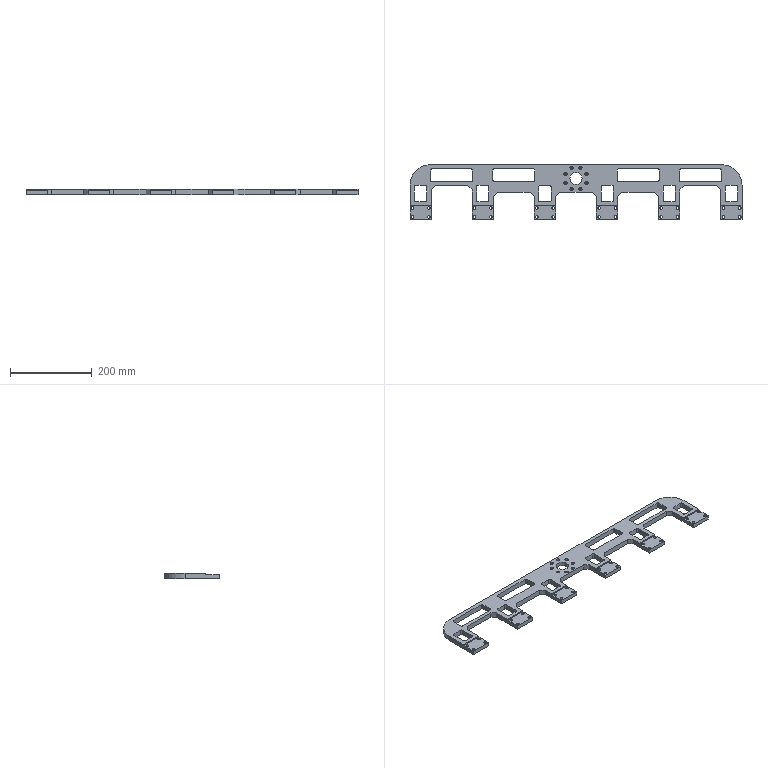NC program | NX | posted with a generic post | part box 813.6 x 134 x 13 mm
Lines 122 to 1297 of 6062:
(ZLEVEL_PROFILE_COPY_3_COPY_1 , TOOL : D10)
N224 T10 M6
N226 G54
N228 G17 G0 G90 X-398.181 Y53.373 S9500 M3
N230 G43 Z30. H10
N232 Z1.5
N234 G94 G1 X-396.785 Y54.925 Z1.391 F1000.
N236 X-394.725 Y56.985 Z1.238
N238 X-392.56 Y58.932 Z1.085
N240 X-390.295 Y60.763 Z0.933
N242 X-387.936 Y62.471 Z0.78
N244 X-385.491 Y64.053 Z0.627
N246 X-382.965 Y65.503 Z0.475
N248 X-380.366 Y66.817 Z0.322
N250 X-377.702 Y67.992 Z0.17
N252 X-374.979 Y69.025 Z0.017
N254 X-372.205 Y69.913 Z-0.136
N256 X-369.388 Y70.653 Z-0.288
N258 X-366.536 Y71.243 Z-0.441
N260 X-363.657 Y71.682 Z-0.594
N262 X-360.759 Y71.968 Z-0.746
N264 X-357.85 Y72.1 Z-0.899
N266 X-356.8 Z-0.954
N268 X356.801 F3500.
N270 G2 X411.9 Y16.999 R55.1
N272 G1 Y-67.
N274 G2 X406.8 Y-72.1 R5.1
N276 G1 X354.8
N278 G2 X349.7 Y-67. R5.1
N280 G1 Y2.888
N282 X342.687 Y9.9
N284 X266.913
N286 X259.9 Y2.888
N288 Y-67.
N290 G2 X254.8 Y-72.1 R5.1
N292 G1 X202.4
N294 G2 X197.3 Y-67. R5.1
N296 G1 Y-13.062
N298 X190.288 Y-6.05
N300 X114.512
N302 X107.5 Y-13.062
N304 Y-67.
N306 G2 X102.4 Y-72.1 R5.1
N308 G1 X50.
N310 G2 X44.9 Y-67. R5.1
N312 G1 Y-13.062
N314 X37.888 Y-6.05
N316 X-37.888
N318 X-44.9 Y-13.062
N320 Y-67.
N322 G2 X-50. Y-72.1 R5.1
N324 G1 X-102.4
N326 G2 X-107.5 Y-67. R5.1
N328 G1 Y-13.062
N330 X-114.512 Y-6.05
N332 X-190.288
N334 X-197.3 Y-13.062
N336 Y-67.
N338 G2 X-202.4 Y-72.1 R5.1
N340 G1 X-254.8
N342 G2 X-259.9 Y-67. R5.1
N344 G1 Y2.888
N346 X-266.913 Y9.9
N348 X-342.687
N350 X-349.7 Y2.888
N352 Y-67.
N354 G2 X-354.8 Y-72.1 R5.1
N356 G1 X-406.8
N358 G2 X-411.9 Y-67. R5.1
N360 G1 Y17.
N362 G2 X-356.8 Y72.1 R55.1
N364 G1 X-302.154 Z-1.908
N366 X356.801
N368 G2 X411.9 Y16.999 R55.1
N370 G1 Y-67.
N372 G2 X406.8 Y-72.1 R5.1
N374 G1 X354.8
N376 G2 X349.7 Y-67. R5.1
N378 G1 Y2.888
N380 X342.687 Y9.9
N382 X266.913
N384 X259.9 Y2.888
N386 Y-67.
N388 G2 X254.8 Y-72.1 R5.1
N390 G1 X202.4
N392 G2 X197.3 Y-67. R5.1
N394 G1 Y-13.062
N396 X190.288 Y-6.05
N398 X114.512
N400 X107.5 Y-13.062
N402 Y-67.
N404 G2 X102.4 Y-72.1 R5.1
N406 G1 X50.
N408 G2 X44.9 Y-67. R5.1
N410 G1 Y-13.062
N412 X37.888 Y-6.05
N414 X-37.888
N416 X-44.9 Y-13.062
N418 Y-67.
N420 G2 X-50. Y-72.1 R5.1
N422 G1 X-102.4
N424 G2 X-107.5 Y-67. R5.1
N426 G1 Y-13.062
N428 X-114.512 Y-6.05
N430 X-190.288
N432 X-197.3 Y-13.062
N434 Y-67.
N436 G2 X-202.4 Y-72.1 R5.1
N438 G1 X-254.8
N440 G2 X-259.9 Y-67. R5.1
N442 G1 Y2.888
N444 X-266.913 Y9.9
N446 X-342.687
N448 X-349.7 Y2.888
N450 Y-67.
N452 G2 X-354.8 Y-72.1 R5.1
N454 G1 X-406.8
N456 G2 X-411.9 Y-67. R5.1
N458 G1 Y17.
N460 G2 X-356.8 Y72.1 R55.1
N462 G1 X-302.154 Z-2.862
N464 X356.801
N466 G2 X411.9 Y16.999 R55.1
N468 G1 Y-67.
N470 G2 X406.8 Y-72.1 R5.1
N472 G1 X354.8
N474 G2 X349.7 Y-67. R5.1
N476 G1 Y2.888
N478 X342.687 Y9.9
N480 X266.913
N482 X259.9 Y2.888
N484 Y-67.
N486 G2 X254.8 Y-72.1 R5.1
N488 G1 X202.4
N490 G2 X197.3 Y-67. R5.1
N492 G1 Y-13.062
N494 X190.288 Y-6.05
N496 X114.512
N498 X107.5 Y-13.062
N500 Y-67.
N502 G2 X102.4 Y-72.1 R5.1
N504 G1 X50.
N506 G2 X44.9 Y-67. R5.1
N508 G1 Y-13.062
N510 X37.888 Y-6.05
N512 X-37.888
N514 X-44.9 Y-13.062
N516 Y-67.
N518 G2 X-50. Y-72.1 R5.1
N520 G1 X-102.4
N522 G2 X-107.5 Y-67. R5.1
N524 G1 Y-13.062
N526 X-114.512 Y-6.05
N528 X-190.288
N530 X-197.3 Y-13.062
N532 Y-67.
N534 G2 X-202.4 Y-72.1 R5.1
N536 G1 X-254.8
N538 G2 X-259.9 Y-67. R5.1
N540 G1 Y2.888
N542 X-266.913 Y9.9
N544 X-342.687
N546 X-349.7 Y2.888
N548 Y-67.
N550 G2 X-354.8 Y-72.1 R5.1
N552 G1 X-406.8
N554 G2 X-411.9 Y-67. R5.1
N556 G1 Y17.
N558 G2 X-356.8 Y72.1 R55.1
N560 G1 X-302.154 Z-3.815
N562 X356.801
N564 G2 X411.9 Y16.999 R55.1
N566 G1 Y-67.
N568 G2 X406.8 Y-72.1 R5.1
N570 G1 X354.8
N572 G2 X349.7 Y-67. R5.1
N574 G1 Y2.888
N576 X342.687 Y9.9
N578 X266.913
N580 X259.9 Y2.888
N582 Y-67.
N584 G2 X254.8 Y-72.1 R5.1
N586 G1 X202.4
N588 G2 X197.3 Y-67. R5.1
N590 G1 Y-13.062
N592 X190.288 Y-6.05
N594 X114.512
N596 X107.5 Y-13.062
N598 Y-67.
N600 G2 X102.4 Y-72.1 R5.1
N602 G1 X50.
N604 G2 X44.9 Y-67. R5.1
N606 G1 Y-13.062
N608 X37.888 Y-6.05
N610 X-37.888
N612 X-44.9 Y-13.062
N614 Y-67.
N616 G2 X-50. Y-72.1 R5.1
N618 G1 X-102.4
N620 G2 X-107.5 Y-67. R5.1
N622 G1 Y-13.062
N624 X-114.512 Y-6.05
N626 X-190.288
N628 X-197.3 Y-13.062
N630 Y-67.
N632 G2 X-202.4 Y-72.1 R5.1
N634 G1 X-254.8
N636 G2 X-259.9 Y-67. R5.1
N638 G1 Y2.888
N640 X-266.913 Y9.9
N642 X-342.687
N644 X-349.7 Y2.888
N646 Y-67.
N648 G2 X-354.8 Y-72.1 R5.1
N650 G1 X-406.8
N652 G2 X-411.9 Y-67. R5.1
N654 G1 Y17.
N656 G2 X-356.8 Y72.1 R55.1
N658 G1 X-302.154 Z-4.769
N660 X356.801
N662 G2 X411.9 Y16.999 R55.1
N664 G1 Y-67.
N666 G2 X406.8 Y-72.1 R5.1
N668 G1 X354.8
N670 G2 X349.7 Y-67. R5.1
N672 G1 Y2.888
N674 X342.687 Y9.9
N676 X266.913
N678 X259.9 Y2.888
N680 Y-67.
N682 G2 X254.8 Y-72.1 R5.1
N684 G1 X202.4
N686 G2 X197.3 Y-67. R5.1
N688 G1 Y-13.062
N690 X190.288 Y-6.05
N692 X114.512
N694 X107.5 Y-13.062
N696 Y-67.
N698 G2 X102.4 Y-72.1 R5.1
N700 G1 X50.
N702 G2 X44.9 Y-67. R5.1
N704 G1 Y-13.062
N706 X37.888 Y-6.05
N708 X-37.888
N710 X-44.9 Y-13.062
N712 Y-67.
N714 G2 X-50. Y-72.1 R5.1
N716 G1 X-102.4
N718 G2 X-107.5 Y-67. R5.1
N720 G1 Y-13.062
N722 X-114.512 Y-6.05
N724 X-190.288
N726 X-197.3 Y-13.062
N728 Y-67.
N730 G2 X-202.4 Y-72.1 R5.1
N732 G1 X-254.8
N734 G2 X-259.9 Y-67. R5.1
N736 G1 Y2.888
N738 X-266.913 Y9.9
N740 X-342.687
N742 X-349.7 Y2.888
N744 Y-67.
N746 G2 X-354.8 Y-72.1 R5.1
N748 G1 X-406.8
N750 G2 X-411.9 Y-67. R5.1
N752 G1 Y17.
N754 G2 X-356.8 Y72.1 R55.1
N756 G1 X-302.154 Z-5.723
N758 X356.801
N760 G2 X411.9 Y16.999 R55.1
N762 G1 Y-67.
N764 G2 X406.8 Y-72.1 R5.1
N766 G1 X354.8
N768 G2 X349.7 Y-67. R5.1
N770 G1 Y2.888
N772 X342.687 Y9.9
N774 X266.913
N776 X259.9 Y2.888
N778 Y-67.
N780 G2 X254.8 Y-72.1 R5.1
N782 G1 X202.4
N784 G2 X197.3 Y-67. R5.1
N786 G1 Y-13.062
N788 X190.288 Y-6.05
N790 X114.512
N792 X107.5 Y-13.062
N794 Y-67.
N796 G2 X102.4 Y-72.1 R5.1
N798 G1 X50.
N800 G2 X44.9 Y-67. R5.1
N802 G1 Y-13.062
N804 X37.888 Y-6.05
N806 X-37.888
N808 X-44.9 Y-13.062
N810 Y-67.
N812 G2 X-50. Y-72.1 R5.1
N814 G1 X-102.4
N816 G2 X-107.5 Y-67. R5.1
N818 G1 Y-13.062
N820 X-114.512 Y-6.05
N822 X-190.288
N824 X-197.3 Y-13.062
N826 Y-67.
N828 G2 X-202.4 Y-72.1 R5.1
N830 G1 X-254.8
N832 G2 X-259.9 Y-67. R5.1
N834 G1 Y2.888
N836 X-266.913 Y9.9
N838 X-342.687
N840 X-349.7 Y2.888
N842 Y-67.
N844 G2 X-354.8 Y-72.1 R5.1
N846 G1 X-406.8
N848 G2 X-411.9 Y-67. R5.1
N850 G1 Y17.
N852 G2 X-356.8 Y72.1 R55.1
N854 G1 X-302.154 Z-6.677
N856 X356.801
N858 G2 X411.9 Y16.999 R55.1
N860 G1 Y-67.
N862 G2 X406.8 Y-72.1 R5.1
N864 G1 X354.8
N866 G2 X349.7 Y-67. R5.1
N868 G1 Y2.888
N870 X342.687 Y9.9
N872 X266.913
N874 X259.9 Y2.888
N876 Y-67.
N878 G2 X254.8 Y-72.1 R5.1
N880 G1 X202.4
N882 G2 X197.3 Y-67. R5.1
N884 G1 Y-13.062
N886 X190.288 Y-6.05
N888 X114.512
N890 X107.5 Y-13.062
N892 Y-67.
N894 G2 X102.4 Y-72.1 R5.1
N896 G1 X50.
N898 G2 X44.9 Y-67. R5.1
N900 G1 Y-13.062
N902 X37.888 Y-6.05
N904 X-37.888
N906 X-44.9 Y-13.062
N908 Y-67.
N910 G2 X-50. Y-72.1 R5.1
N912 G1 X-102.4
N914 G2 X-107.5 Y-67. R5.1
N916 G1 Y-13.062
N918 X-114.512 Y-6.05
N920 X-190.288
N922 X-197.3 Y-13.062
N924 Y-67.
N926 G2 X-202.4 Y-72.1 R5.1
N928 G1 X-254.8
N930 G2 X-259.9 Y-67. R5.1
N932 G1 Y2.888
N934 X-266.913 Y9.9
N936 X-342.687
N938 X-349.7 Y2.888
N940 Y-67.
N942 G2 X-354.8 Y-72.1 R5.1
N944 G1 X-406.8
N946 G2 X-411.9 Y-67. R5.1
N948 G1 Y17.
N950 G2 X-356.8 Y72.1 R55.1
N952 G1 X-302.154 Z-7.631
N954 X356.801
N956 G2 X411.9 Y16.999 R55.1
N958 G1 Y-67.
N960 G2 X406.8 Y-72.1 R5.1
N962 G1 X354.8
N964 G2 X349.7 Y-67. R5.1
N966 G1 Y2.888
N968 X342.687 Y9.9
N970 X266.913
N972 X259.9 Y2.888
N974 Y-67.
N976 G2 X254.8 Y-72.1 R5.1
N978 G1 X202.4
N980 G2 X197.3 Y-67. R5.1
N982 G1 Y-13.062
N984 X190.288 Y-6.05
N986 X114.512
N988 X107.5 Y-13.062
N990 Y-67.
N992 G2 X102.4 Y-72.1 R5.1
N994 G1 X50.
N996 G2 X44.9 Y-67. R5.1
N998 G1 Y-13.062
N1000 X37.888 Y-6.05
N1002 X-37.888
N1004 X-44.9 Y-13.062
N1006 Y-67.
N1008 G2 X-50. Y-72.1 R5.1
N1010 G1 X-102.4
N1012 G2 X-107.5 Y-67. R5.1
N1014 G1 Y-13.062
N1016 X-114.512 Y-6.05
N1018 X-190.288
N1020 X-197.3 Y-13.062
N1022 Y-67.
N1024 G2 X-202.4 Y-72.1 R5.1
N1026 G1 X-254.8
N1028 G2 X-259.9 Y-67. R5.1
N1030 G1 Y2.888
N1032 X-266.913 Y9.9
N1034 X-342.687
N1036 X-349.7 Y2.888
N1038 Y-67.
N1040 G2 X-354.8 Y-72.1 R5.1
N1042 G1 X-406.8
N1044 G2 X-411.9 Y-67. R5.1
N1046 G1 Y17.
N1048 G2 X-356.8 Y72.1 R55.1
N1050 G1 X-302.376 Z-8.581
N1052 X-302.154 Z-8.585
N1054 X356.801
N1056 G2 X411.9 Y16.999 R55.1
N1058 G1 Y-67.
N1060 G2 X406.8 Y-72.1 R5.1
N1062 G1 X354.8
N1064 G2 X349.7 Y-67. R5.1
N1066 G1 Y2.888
N1068 X342.688 Y9.9
N1070 X266.912
N1072 X259.9 Y2.888
N1074 Y-67.
N1076 G2 X254.8 Y-72.1 R5.1
N1078 G1 X202.4
N1080 G2 X197.3 Y-67. R5.1
N1082 G1 Y-13.062
N1084 X190.288 Y-6.05
N1086 X114.512
N1088 X107.5 Y-13.062
N1090 Y-67.
N1092 G2 X102.4 Y-72.1 R5.1
N1094 G1 X50.
N1096 G2 X44.9 Y-67. R5.1
N1098 G1 Y-13.062
N1100 X37.888 Y-6.05
N1102 X-37.888
N1104 X-44.9 Y-13.062
N1106 Y-67.
N1108 G2 X-50. Y-72.1 R5.1
N1110 G1 X-102.4
N1112 G2 X-107.5 Y-67. R5.1
N1114 G1 Y-13.062
N1116 X-114.512 Y-6.05
N1118 X-190.288
N1120 X-197.3 Y-13.062
N1122 Y-67.
N1124 G2 X-202.4 Y-72.1 R5.1
N1126 G1 X-254.8
N1128 G2 X-259.9 Y-67. R5.1
N1130 G1 Y2.888
N1132 X-266.912 Y9.9
N1134 X-342.688
N1136 X-349.7 Y2.888
N1138 Y-67.
N1140 G2 X-354.8 Y-72.1 R5.1
N1142 G1 X-406.8
N1144 G2 X-411.9 Y-67. R5.1
N1146 G1 Y17.
N1148 G2 X-356.8 Y72.1 R55.1
N1150 G1 X-356.578 Z-8.588
N1152 X-302.376 Z-9.535
N1154 X-302.154 Z-9.538
N1156 X356.801
N1158 G2 X411.9 Y16.999 R55.1
N1160 G1 Y-67.
N1162 G2 X406.8 Y-72.1 R5.1
N1164 G1 X354.8
N1166 G2 X349.7 Y-67. R5.1
N1168 G1 Y2.888
N1170 X342.688 Y9.9
N1172 X266.912
N1174 X259.9 Y2.888
N1176 Y-67.
N1178 G2 X254.8 Y-72.1 R5.1
N1180 G1 X202.4
N1182 G2 X197.3 Y-67. R5.1
N1184 G1 Y-13.062
N1186 X190.288 Y-6.05
N1188 X114.512
N1190 X107.5 Y-13.062
N1192 Y-67.
N1194 G2 X102.4 Y-72.1 R5.1
N1196 G1 X50.
N1198 G2 X44.9 Y-67. R5.1
N1200 G1 Y-13.062
N1202 X37.888 Y-6.05
N1204 X-37.888
N1206 X-44.9 Y-13.062
N1208 Y-67.
N1210 G2 X-50. Y-72.1 R5.1
N1212 G1 X-102.4
N1214 G2 X-107.5 Y-67. R5.1
N1216 G1 Y-13.062
N1218 X-114.512 Y-6.05
N1220 X-190.288
N1222 X-197.3 Y-13.062
N1224 Y-67.
N1226 G2 X-202.4 Y-72.1 R5.1
N1228 G1 X-254.8
N1230 G2 X-259.9 Y-67. R5.1
N1232 G1 Y2.888
N1234 X-266.912 Y9.9
N1236 X-342.688
N1238 X-349.7 Y2.888
N1240 Y-67.
N1242 G2 X-354.8 Y-72.1 R5.1
N1244 G1 X-406.8
N1246 G2 X-411.9 Y-67. R5.1
N1248 G1 Y17.
N1250 G2 X-356.8 Y72.1 R55.1
N1252 G1 X-356.578 Z-9.542
N1254 X-302.376 Z-10.488
N1256 X-302.154 Z-10.492
N1258 X356.801
N1260 G2 X411.9 Y16.999 R55.1
N1262 G1 Y-67.
N1264 G2 X406.8 Y-72.1 R5.1
N1266 G1 X354.8
N1268 G2 X349.7 Y-67. R5.1
N1270 G1 Y2.888
N1272 X342.688 Y9.9
N1274 X266.912
N1276 X259.9 Y2.888
N1278 Y-67.
N1280 G2 X254.8 Y-72.1 R5.1
N1282 G1 X202.4
N1284 G2 X197.3 Y-67. R5.1
N1286 G1 Y-13.062
N1288 X190.288 Y-6.05
N1290 X114.512
N1292 X107.5 Y-13.062
N1294 Y-67.
N1296 G2 X102.4 Y-72.1 R5.1
N1298 G1 X50.
N1300 G2 X44.9 Y-67. R5.1
N1302 G1 Y-13.062
N1304 X37.888 Y-6.05
N1306 X-37.888
N1308 X-44.9 Y-13.062
N1310 Y-67.
N1312 G2 X-50. Y-72.1 R5.1
N1314 G1 X-102.4
N1316 G2 X-107.5 Y-67. R5.1
N1318 G1 Y-13.062
N1320 X-114.512 Y-6.05
N1322 X-190.288
N1324 X-197.3 Y-13.062
N1326 Y-67.
N1328 G2 X-202.4 Y-72.1 R5.1
N1330 G1 X-254.8
N1332 G2 X-259.9 Y-67. R5.1
N1334 G1 Y2.888
N1336 X-266.912 Y9.9
N1338 X-342.688
N1340 X-349.7 Y2.888
N1342 Y-67.
N1344 G2 X-354.8 Y-72.1 R5.1
N1346 G1 X-406.8
N1348 G2 X-411.9 Y-67. R5.1
N1350 G1 Y17.
N1352 G2 X-356.8 Y72.1 R55.1
N1354 G1 X-356.578 Z-10.496
N1356 X-302.376 Z-11.442
N1358 X-302.154 Z-11.446
N1360 X356.801
N1362 G2 X411.9 Y16.999 R55.1
N1364 G1 Y-67.
N1366 G2 X406.8 Y-72.1 R5.1
N1368 G1 X354.8
N1370 G2 X349.7 Y-67. R5.1
N1372 G1 Y2.888
N1374 X342.688 Y9.9
N1376 X266.912
N1378 X259.9 Y2.888
N1380 Y-67.
N1382 G2 X254.8 Y-72.1 R5.1
N1384 G1 X202.4
N1386 G2 X197.3 Y-67. R5.1
N1388 G1 Y-13.062
N1390 X190.288 Y-6.05
N1392 X114.512
N1394 X107.5 Y-13.062
N1396 Y-67.
N1398 G2 X102.4 Y-72.1 R5.1
N1400 G1 X50.
N1402 G2 X44.9 Y-67. R5.1
N1404 G1 Y-13.062
N1406 X37.888 Y-6.05
N1408 X-37.888
N1410 X-44.9 Y-13.062
N1412 Y-67.
N1414 G2 X-50. Y-72.1 R5.1
N1416 G1 X-102.4
N1418 G2 X-107.5 Y-67. R5.1
N1420 G1 Y-13.062
N1422 X-114.512 Y-6.05
N1424 X-190.288
N1426 X-197.3 Y-13.062
N1428 Y-67.
N1430 G2 X-202.4 Y-72.1 R5.1
N1432 G1 X-254.8
N1434 G2 X-259.9 Y-67. R5.1
N1436 G1 Y2.888
N1438 X-266.912 Y9.9
N1440 X-342.688
N1442 X-349.7 Y2.888
N1444 Y-67.
N1446 G2 X-354.8 Y-72.1 R5.1
N1448 G1 X-406.8
N1450 G2 X-411.9 Y-67. R5.1
N1452 G1 Y17.
N1454 G2 X-356.8 Y72.1 R55.1
N1456 G1 X-356.578 Z-11.45
N1458 X-302.376 Z-12.396
N1460 X-302.154 Z-12.4
N1462 X356.801
N1464 G2 X411.9 Y16.999 R55.1
N1466 G1 Y-67.
N1468 G2 X406.8 Y-72.1 R5.1
N1470 G1 X354.8
N1472 G2 X349.7 Y-67. R5.1
N1474 G1 Y2.888
N1476 X342.688 Y9.9
N1478 X266.912
N1480 X259.9 Y2.888
N1482 Y-67.
N1484 G2 X254.8 Y-72.1 R5.1
N1486 G1 X202.4
N1488 G2 X197.3 Y-67. R5.1
N1490 G1 Y-13.062
N1492 X190.288 Y-6.05
N1494 X114.512
N1496 X107.5 Y-13.062
N1498 Y-67.
N1500 G2 X102.4 Y-72.1 R5.1
N1502 G1 X50.
N1504 G2 X44.9 Y-67. R5.1
N1506 G1 Y-13.062
N1508 X37.888 Y-6.05
N1510 X-37.888
N1512 X-44.9 Y-13.062
N1514 Y-67.
N1516 G2 X-50. Y-72.1 R5.1
N1518 G1 X-102.4
N1520 G2 X-107.5 Y-67. R5.1
N1522 G1 Y-13.062
N1524 X-114.512 Y-6.05
N1526 X-190.288
N1528 X-197.3 Y-13.062
N1530 Y-67.
N1532 G2 X-202.4 Y-72.1 R5.1
N1534 G1 X-254.8
N1536 G2 X-259.9 Y-67. R5.1
N1538 G1 Y2.888
N1540 X-266.912 Y9.9
N1542 X-342.688
N1544 X-349.7 Y2.888
N1546 Y-67.
N1548 G2 X-354.8 Y-72.1 R5.1
N1550 G1 X-406.8
N1552 G2 X-411.9 Y-67. R5.1
N1554 G1 Y17.
N1556 G2 X-356.8 Y72.1 R55.1
N1558 G1 X-302.154
N1560 Z-10.9
N1562 G0 Z30.
(HOLE_MILLING , TOOL : D10)
N1564 X0. Y33. S8500
N1566 Z1.
N1568 G3 X-1.25 Y34.25 R1.25 F2000.
N1570 X-2.5 Y33. R1.25
N1572 X-2.5 Y33. Z0. I2.5 J0.
N1574 X-2.5 Y33. Z-1. I2.5 J0.
N1576 X-2.5 Y33. Z-2. I2.5 J0.
N1578 X-2.5 Y33. Z-3. I2.5 J0.
N1580 X0.112 Y30.322 R2.679
N1582 X2.99 Y32.863 R2.821
N1584 X0.289 Y36.223 R3.078
N1586 X-3.471 Y33.319 R3.392
N1588 X-0.493 Y29.303 R3.571
N1590 X3.941 Y32.455 R3.886
N1592 X0.74 Y37.157 R4.064
N1594 X-4.396 Y33.815 R4.379
N1596 X-1.031 Y28.399 R4.557
N1598 X4.834 Y31.873 R4.872
N1600 X1.363 Y38.027 R5.05
N1602 X-5.251 Y34.481 R5.365
N1604 X-1.736 Y27.57 R5.543
N1606 X5.646 Y31.125 R5.857
N1608 X2.149 Y38.809 R6.036
N1610 X-6.014 Y35.308 R6.35
N1612 X-2.6 Y26.839 R6.529
N1614 X6.353 Y30.221 R6.843
N1616 X3.087 Y39.482 R7.022
N1618 X-6.661 Y36.285 R7.336
N1620 X-3.609 Y26.229 R7.515
N1622 X6.935 Y29.176 R7.829
N1624 X4.163 Y40.024 R8.008
N1626 X-7.173 Y37.396 R8.322
N1628 X-4.747 Y25.76 R8.5
N1630 X7.372 Y28.004 R8.814
N1632 X5.36 Y40.417 R8.993
N1634 X-7.53 Y38.623 R9.307
N1636 X-5.997 Y25.448 R9.486
N1638 X7.646 Y26.725 R9.8
N1640 X6.658 Y40.643 R9.979
N1642 X-7.716 Y39.948 R10.293
N1644 X-7.339 Y25.312 R10.471
N1646 X7.741 Y25.36 R10.786
N1648 X8.038 Y40.687 R10.964
N1650 X-7.717 Y41.348 R11.278
N1652 X-8.751 Y25.363 R11.457
N1654 X7.644 Y23.93 R11.771
N1656 X9.475 Y40.537 R11.95
N1658 X-7.521 Y42.801 R12.264
N1660 X-10.208 Y25.614 R12.442
N1662 X7.346 Y22.46 R12.757
N1664 X10.946 Y40.183 R12.935
N1666 X-7.118 Y44.282 R13.249
N1668 X-11.686 Y26.073 R13.428
N1670 X6.838 Y20.976 R13.742
N1672 X12.425 Y39.618 R13.921
N1674 X-6.503 Y45.764 R14.235
N1676 X-13.159 Y26.744 R14.413
N1678 X6.115 Y19.503 R14.728
N1680 X13.885 Y38.84 R14.906
N1682 X-5.673 Y47.22 R15.22
N1684 X-14.6 Y27.63 R15.399
N1686 X5.178 Y18.069 R15.713
N1688 X15.3 Y37.846 R15.892
N1690 X-4.628 Y48.625 R16.206
N1692 X-15.981 Y28.73 R16.384
N1694 X4.026 Y16.701 R16.698
N1696 X16.641 Y36.64 R16.877
N1698 X-3.371 Y49.949 R17.191
N1700 X-17.275 Y30.041 R17.37
N1702 X2.666 Y15.427 R17.684
N1704 X17.882 Y35.228 R17.863
N1706 X-1.909 Y51.167 R18.177
N1708 X-18.456 Y31.553 R18.355
N1710 X1.104 Y14.273 R18.669
N1712 X18.995 Y33.618 R18.848
N1714 X-0.252 Y52.25 R19.162
N1716 X-19.496 Y33.258 R19.341
N1718 X-0.646 Y13.266 R19.655
N1720 X19.956 Y31.822 R19.833
N1722 X1.588 Y53.175 R20.148
N1724 X-20.371 Y35.14 R20.326
N1726 X-2.571 Y12.43 R20.64
N1728 X20.739 Y29.857 R20.819
N1730 X3.594 Y53.916 R21.133
N1732 X-21.057 Y37.184 R21.312
N1734 X-4.654 Y11.789 R21.626
N1736 X21.322 Y27.739 R21.804
N1738 X5.748 Y54.452 R22.118
N1740 X-21.532 Y39.37 R22.297
N1742 X-6.874 Y11.365 R22.611
N1744 X21.683 Y25.49 R22.79
N1746 X8.028 Y54.76 R23.104
N1748 X-21.775 Y41.676 R23.282
N1750 X-9.207 Y11.176 R23.597
N1752 X21.804 Y23.134 R23.775
N1754 X10.409 Y54.824 R24.089
N1756 X-21.769 Y44.077 R24.268
N1758 X-11.63 Y11.241 R24.582
N1760 X21.668 Y20.696 R24.761
N1762 X12.866 Y54.627 R25.075
N1764 X-21.499 Y46.545 R25.253
N1766 X-14.114 Y11.574 R25.568
N1768 X21.459 Y18.35 R25.826
N1770 X15.371 Y54.156 R25.978
N1772 X-21.156 Y48.371 R26.15
N1774 X15.371 Y54.156 R-26.15
N1776 X-2.893 Y51.263 R13.075
N1778 X0. Y33. R13.075
N1780 G0 Z30.
(FLOOR_WALL_1_COPY_COPY_COPY , TOOL : D10)
N1782 X0.866 Y58.15 S9500
N1784 Z-1.5
N1786 G1 Z-3. F1000.
N1788 G3 X0. Y58.65 R1.
N1790 G2 X25.65 Y33. R25.65 F1500.
N1792 X0. Y58.65 R-25.65
N1794 G1 Y52.65
N1796 G2 X19.65 Y33. R19.65
N1798 X0. Y52.65 R-19.65
N1800 G1 Y46.65
N1802 G2 X13.65 Y33. R13.65
N1804 X0. Y46.65 R-13.65
N1806 G1 Y40.65
N1808 G2 X7.65 Y33. R7.65
N1810 X0. Y40.65 R-7.65
N1812 G1 Y34.65
N1814 G2 X1.65 Y33. R1.65
N1816 X0. Y34.65 R-1.65
N1818 G3 X0.866 Y35.15 R1.
N1820 G1 Z-1.5
N1822 X0.993 Y58.431 F800.
N1824 Z-3. F1000.
N1826 X0.866 Y58.65
N1828 G3 X0. Y59.15 R1.
N1830 X-26.15 Y33. R26.15 F1500.
N1832 X0. Y59.15 R-26.15
N1834 X-0.866 Y58.65 R1.
N1836 G1 Z-1.5
N1838 G0 Z30.
(ZLEVEL_PROFILE_COPY_2_COPY_COPY , TOOL : D10)
N1840 X350.7 Y50.246
N1842 Z1.5
N1844 G1 Y51.902 Z1.413 F1000.
N1846 X350.662 Y51.9 Z1.411
N1848 X304.8 Z-0.992
N1850 X258.954 F3500.
N1852 X258.9 Y51.902
N1854 Y30.1
N1856 X350.7
N1858 Y51.902
N1860 X350.662 Y51.9
N1862 X304.8
N1864 X259.054 Z-1.791
N1866 X258.9 Z-1.794
N1868 Y51.612 Z-1.799
N1870 Y40.953 Z-1.985
N1872 Y30.1
N1874 X350.7
N1876 Y51.902
N1878 X350.662 Y51.9
N1880 X304.8
N1882 X259.054 Z-2.783
N1884 X258.9 Z-2.786
N1886 Y51.612 Z-2.791
N1888 Y40.953 Z-2.977
N1890 Y30.1
N1892 X350.7
N1894 Y51.902
N1896 X350.662 Y51.9
N1898 X304.8
N1900 X259.054 Z-3.775
N1902 X258.9 Z-3.778
N1904 Y51.612 Z-3.783
N1906 Y40.953 Z-3.969
N1908 Y30.1
N1910 X350.7
N1912 Y51.902
N1914 X350.662 Y51.9
N1916 X304.8
N1918 X259.054 Z-4.768
N1920 X258.9 Z-4.77
N1922 Y51.612 Z-4.775
N1924 Y40.953 Z-4.962
N1926 Y30.1
N1928 X350.7
N1930 Y51.902
N1932 X350.662 Y51.9
N1934 X304.8
N1936 X259.054 Z-5.76
N1938 X258.9 Z-5.763
N1940 Y51.612 Z-5.768
N1942 Y40.953 Z-5.954
N1944 Y30.1
N1946 X350.7
N1948 Y51.902
N1950 X350.662 Y51.9
N1952 X304.8
N1954 X259.054 Z-6.752
N1956 X258.9 Z-6.755
N1958 Y51.612 Z-6.76
N1960 Y40.953 Z-6.946
N1962 Y30.1
N1964 X350.7
N1966 Y51.902
N1968 X350.662 Y51.9
N1970 X304.8
N1972 X259.054 Z-7.745
N1974 X258.9 Z-7.747
N1976 Y51.612 Z-7.752
N1978 Y40.953 Z-7.938
N1980 Y30.1
N1982 X350.7
N1984 Y51.902
N1986 X350.662 Y51.9
N1988 X304.8
N1990 X259.054 Z-8.737
N1992 X258.9 Z-8.74
N1994 Y51.612 Z-8.745
N1996 Y40.953 Z-8.931
N1998 Y30.1
N2000 X350.7
N2002 Y51.902
N2004 X350.662 Y51.9
N2006 X304.8
N2008 X259.054 Z-9.729
N2010 X258.9 Z-9.732
N2012 Y51.612 Z-9.737
N2014 Y40.953 Z-9.923
N2016 Y30.1
N2018 X350.7
N2020 Y51.902
N2022 X350.662 Y51.9
N2024 X304.8
N2026 X259.054 Z-10.722
N2028 X258.9 Z-10.724
N2030 Y51.612 Z-10.729
N2032 Y40.953 Z-10.915
N2034 Y30.1
N2036 X350.7
N2038 Y51.902
N2040 X350.662 Y51.9
N2042 X304.8
N2044 X259.054 Z-11.714
N2046 X258.9 Z-11.717
N2048 Y51.612 Z-11.722
N2050 Y40.953 Z-11.908
N2052 Y30.1
N2054 X350.7
N2056 Y51.902
N2058 X350.662 Y51.9
N2060 X304.8
N2062 X259.054 Z-12.706
N2064 X258.9 Z-12.709
N2066 Y51.612 Z-12.714
N2068 Y40.953 Z-12.9
N2070 Y30.1
N2072 X350.7
N2074 Y51.902
N2076 X350.662 Y51.9
N2078 X258.954
N2080 X258.9 Y51.902
N2082 Y40.953
N2084 Z-11.4
N2086 G0 Z30.
N2088 X198.3 Y50.247
N2090 Z1.5
N2092 G1 Y51.903 Z1.413 F1000.
N2094 X198.274 Y51.9 Z1.412
N2096 X152.4 Z-0.992
N2098 X106.542 F3500.
N2100 X106.5 Y51.902
N2102 Y30.1
N2104 X198.3
N2106 Y51.903
N2108 X198.274 Y51.9
N2110 X152.4
N2112 X106.654 Z-1.791
N2114 X106.5 Z-1.794
N2116 Y51.612 Z-1.799
N2118 Y40.953 Z-1.985
N2120 Y30.1
N2122 X198.3
N2124 Y51.903
N2126 X198.274 Y51.9
N2128 X152.4
N2130 X106.654 Z-2.783
N2132 X106.5 Z-2.786
N2134 Y51.612 Z-2.791
N2136 Y40.953 Z-2.977
N2138 Y30.1
N2140 X198.3
N2142 Y51.903
N2144 X198.274 Y51.9
N2146 X152.4
N2148 X106.654 Z-3.775
N2150 X106.5 Z-3.778
N2152 Y51.612 Z-3.783
N2154 Y40.953 Z-3.969
N2156 Y30.1
N2158 X198.3
N2160 Y51.903
N2162 X198.274 Y51.9
N2164 X152.4
N2166 X106.654 Z-4.768
N2168 X106.5 Z-4.77
N2170 Y51.612 Z-4.775
N2172 Y40.953 Z-4.962
N2174 Y30.1
N2176 X198.3
N2178 Y51.903
N2180 X198.274 Y51.9
N2182 X152.4
N2184 X106.654 Z-5.76
N2186 X106.5 Z-5.763
N2188 Y51.612 Z-5.768
N2190 Y40.953 Z-5.954
N2192 Y30.1
N2194 X198.3
N2196 Y51.903
N2198 X198.274 Y51.9
N2200 X152.4
N2202 X106.654 Z-6.752
N2204 X106.5 Z-6.755
N2206 Y51.612 Z-6.76
N2208 Y40.953 Z-6.946
N2210 Y30.1
N2212 X198.3
N2214 Y51.903
N2216 X198.274 Y51.9
N2218 X152.4
N2220 X106.654 Z-7.745
N2222 X106.5 Z-7.747
N2224 Y51.612 Z-7.752
N2226 Y40.953 Z-7.938
N2228 Y30.1
N2230 X198.3
N2232 Y51.903
N2234 X198.274 Y51.9
N2236 X152.4
N2238 X106.654 Z-8.737
N2240 X106.5 Z-8.74
N2242 Y51.612 Z-8.745
N2244 Y40.953 Z-8.931
N2246 Y30.1
N2248 X198.3
N2250 Y51.903
N2252 X198.274 Y51.9
N2254 X152.4
N2256 X106.654 Z-9.729
N2258 X106.5 Z-9.732
N2260 Y51.612 Z-9.737
N2262 Y40.953 Z-9.923
N2264 Y30.1
N2266 X198.3
N2268 Y51.903
N2270 X198.274 Y51.9
N2272 X152.4
N2274 X106.654 Z-10.722
N2276 X106.5 Z-10.724
N2278 Y51.612 Z-10.729
N2280 Y40.953 Z-10.915
N2282 Y30.1
N2284 X198.3
N2286 Y51.903
N2288 X198.274 Y51.9
N2290 X152.4
N2292 X106.654 Z-11.714
N2294 X106.5 Z-11.717
N2296 Y51.612 Z-11.722
N2298 Y40.953 Z-11.908
N2300 Y30.1
N2302 X198.3
N2304 Y51.903
N2306 X198.274 Y51.9
N2308 X152.4
N2310 X106.654 Z-12.706
N2312 X106.5 Z-12.709
N2314 Y51.612 Z-12.714
N2316 Y40.953 Z-12.9
N2318 Y30.1
N2320 X198.3
N2322 Y51.903
N2324 X198.274 Y51.9
N2326 X106.542
N2328 X106.5 Y51.902
N2330 Y40.953
N2332 Z-11.4
N2334 G0 Z30.
N2336 X370.9 Y-6.045
N2338 Z1.5
N2340 G1 Y-18.9 Z0.826 F1000.
N2342 X390.7 Z-0.211
N2344 Y-3.999 Z-0.992
N2346 Y10.902 F3500.
N2348 X390.665 Y10.9
N2350 X370.936
N2352 X370.9 Y10.902
N2354 Y-18.9
N2356 X390.7
N2358 Y-3.999
N2360 Y10.658 Z-1.248
N2362 Y10.9 Z-1.252
N2364 X390.501 Z-1.256
N2366 X370.959 Z-1.597
N2368 X370.9 Z-1.598
N2370 Y10.516 Z-1.605
N2372 Y-11.246 Z-1.985
N2374 Y-18.9
N2376 X390.7
N2378 Y-3.999
N2380 Y10.658 Z-2.24
N2382 Y10.9 Z-2.245
N2384 X390.501 Z-2.248
N2386 X370.959 Z-2.589
N2388 X370.9 Z-2.59
N2390 Y10.516 Z-2.597
N2392 Y-11.246 Z-2.977
N2394 Y-18.9
N2396 X390.7
N2398 Y-3.999
N2400 Y10.658 Z-3.233
N2402 Y10.9 Z-3.237
N2404 X390.501 Z-3.241
N2406 X370.959 Z-3.582
N2408 X370.9 Z-3.583
N2410 Y10.516 Z-3.589
N2412 Y-11.246 Z-3.969
N2414 Y-18.9
N2416 X390.7
N2418 Y-3.999
N2420 Y10.658 Z-4.225
N2422 Y10.9 Z-4.229
N2424 X390.501 Z-4.233
N2426 X370.959 Z-4.574
N2428 X370.9 Z-4.575
N2430 Y10.516 Z-4.582
N2432 Y-11.246 Z-4.962
N2434 Y-18.9
N2436 X390.7
N2438 Y-3.999
N2440 Y10.658 Z-5.217
N2442 Y10.9 Z-5.222
N2444 X390.501 Z-5.225
N2446 X370.959 Z-5.566
N2448 X370.9 Z-5.567
N2450 Y10.516 Z-5.574
N2452 Y-11.246 Z-5.954
N2454 Y-18.9
N2456 X390.7
N2458 Y-3.999
N2460 Y10.658 Z-6.21
N2462 Y10.9 Z-6.214
N2464 X390.501 Z-6.217
N2466 X370.959 Z-6.559
N2468 X370.9 Z-6.56
N2470 Y10.516 Z-6.566
N2472 Y-11.246 Z-6.946
N2474 Y-18.9
N2476 X390.7
N2478 Y-3.999
N2480 Y10.658 Z-7.202
N2482 Y10.9 Z-7.206
N2484 X390.501 Z-7.21
N2486 X370.959 Z-7.551
N2488 X370.9 Z-7.552
N2490 Y10.516 Z-7.559
N2492 Y-11.246 Z-7.938
N2494 Y-18.9
N2496 X390.7
N2498 Y-3.999
N2500 Y10.658 Z-8.194
N2502 Y10.9 Z-8.199
N2504 X390.501 Z-8.202
N2506 X370.959 Z-8.543
N2508 X370.9 Z-8.544
N2510 Y10.516 Z-8.551
N2512 Y-11.246 Z-8.931
N2514 Y-18.9
N2516 X390.7
N2518 Y-3.999
N2520 Y10.658 Z-9.187
N2522 Y10.9 Z-9.191
N2524 X390.501 Z-9.194
N2526 X370.959 Z-9.535
N2528 X370.9 Z-9.536
N2530 Y10.516 Z-9.543
N2532 Y-11.246 Z-9.923
N2534 Y-18.9
N2536 X390.7
N2538 Y-3.999
N2540 Y10.658 Z-10.179
N2542 Y10.9 Z-10.183
N2544 X390.501 Z-10.187
N2546 X370.959 Z-10.528
N2548 X370.9 Z-10.529
N2550 Y10.516 Z-10.536